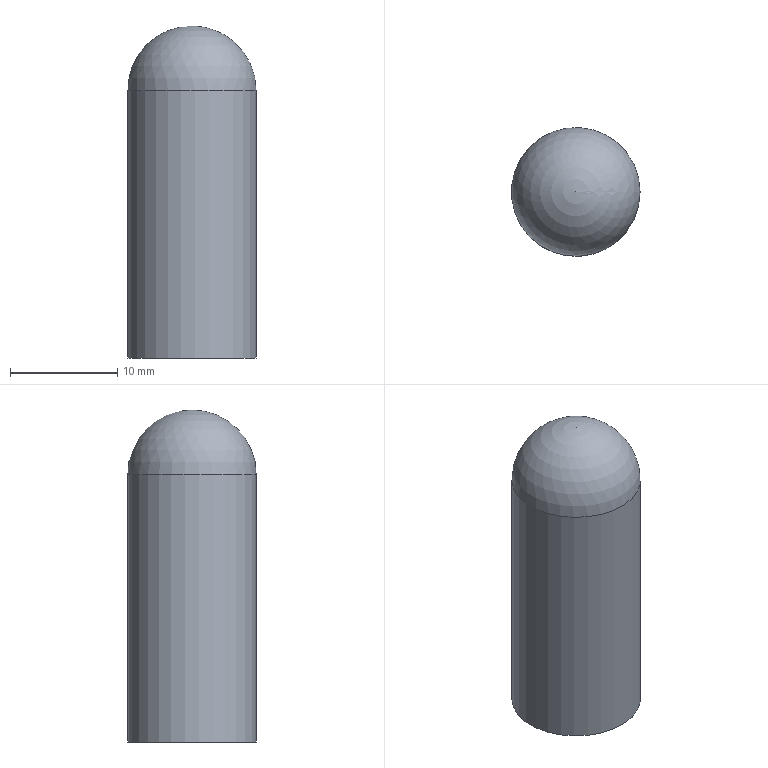Part | NX | features DATUM_CSYS 2, EXTRUDE 1, HOLE PACKAGE 1, SIMPLE HOLE 1, SKETCH 1, SPHERE 1, SYMBOLIC_THREAD 1 | 1 solid | 6 faces | box 12 x 12 x 31 mm | volume 2343 mm3 | cylinder 2 | cone 2 | plane 1 | sphere 1 | commonest cylinder face diameters 6.8 x1 12 x1
STEP:
#1=CARTESIAN_POINT('',(6.,0.,25.));
#2=VERTEX_POINT('',#1);
#3=CARTESIAN_POINT('',(0.,0.,25.));
#4=DIRECTION('',(0.,0.,1.));
#5=DIRECTION('',(1.,0.,0.));
#6=AXIS2_PLACEMENT_3D('',#3,#4,#5);
#7=CIRCLE('',#6,6.);
#8=EDGE_CURVE('',#2,#2,#7,.F.);
#9=ORIENTED_EDGE('',*,*,#8,.T.);
#10=EDGE_LOOP('',(#9));
#11=FACE_BOUND('',#10,.T.);
#12=CARTESIAN_POINT('',(6.,0.,0.));
#13=VERTEX_POINT('',#12);
#14=CARTESIAN_POINT('',(0.,0.,0.));
#15=DIRECTION('',(0.,0.,1.));
#16=DIRECTION('',(1.,0.,0.));
#17=AXIS2_PLACEMENT_3D('',#14,#15,#16);
#18=CIRCLE('',#17,6.);
#19=EDGE_CURVE('',#13,#13,#18,.T.);
#20=ORIENTED_EDGE('',*,*,#19,.T.);
#21=EDGE_LOOP('',(#20));
#22=FACE_BOUND('',#21,.T.);
#23=CARTESIAN_POINT('',(0.,0.,25.));
#24=DIRECTION('',(0.,0.,-1.));
#25=DIRECTION('',(-1.,0.,0.));
#26=AXIS2_PLACEMENT_3D('',#23,#24,#25);
#27=CYLINDRICAL_SURFACE('',#26,6.);
#28=ADVANCED_FACE('',(#11,#22),#27,.T.);
#29=CARTESIAN_POINT('',(4.,0.,0.));
#30=VERTEX_POINT('',#29);
#31=CARTESIAN_POINT('',(0.,0.,0.));
#32=DIRECTION('',(0.,0.,1.));
#33=DIRECTION('',(1.,0.,0.));
#34=AXIS2_PLACEMENT_3D('',#31,#32,#33);
#35=CIRCLE('',#34,4.);
#36=EDGE_CURVE('',#30,#30,#35,.T.);
#37=ORIENTED_EDGE('',*,*,#36,.T.);
#38=EDGE_LOOP('',(#37));
#39=FACE_BOUND('',#38,.T.);
#40=ORIENTED_EDGE('',*,*,#19,.F.);
#41=EDGE_LOOP('',(#40));
#42=FACE_BOUND('',#41,.T.);
#43=CARTESIAN_POINT('',(0.,0.,0.));
#44=DIRECTION('',(0.,0.,1.));
#45=DIRECTION('',(1.,0.,0.));
#46=AXIS2_PLACEMENT_3D('',#43,#44,#45);
#47=PLANE('',#46);
#48=ADVANCED_FACE('',(#39,#42),#47,.F.);
#49=ORIENTED_EDGE('',*,*,#8,.F.);
#50=EDGE_LOOP('',(#49));
#51=FACE_BOUND('',#50,.T.);
#52=CARTESIAN_POINT('',(0.,0.,25.));
#53=DIRECTION('',(0.,0.,1.));
#54=DIRECTION('',(1.,0.,0.));
#55=AXIS2_PLACEMENT_3D('',#52,#53,#54);
#56=SPHERICAL_SURFACE('',#55,6.);
#57=ADVANCED_FACE('',(#51),#56,.T.);
#58=CARTESIAN_POINT('',(3.4,0.,25.));
#59=VERTEX_POINT('',#58);
#60=CARTESIAN_POINT('',(0.,0.,25.));
#61=DIRECTION('',(0.,0.,1.));
#62=DIRECTION('',(1.,0.,0.));
#63=AXIS2_PLACEMENT_3D('',#60,#61,#62);
#64=CIRCLE('',#63,3.4);
#65=EDGE_CURVE('',#59,#59,#64,.F.);
#66=ORIENTED_EDGE('',*,*,#65,.T.);
#67=EDGE_LOOP('',(#66));
#68=FACE_BOUND('',#67,.T.);
#69=CARTESIAN_POINT('',(0.,0.,27.043));
#70=VERTEX_POINT('',#69);
#71=VERTEX_LOOP('',#70);
#72=FACE_BOUND('',#71,.T.);
#73=CARTESIAN_POINT('',(0.,0.,25.));
#74=DIRECTION('',(0.,0.,-1.));
#75=DIRECTION('',(-1.,0.,0.));
#76=AXIS2_PLACEMENT_3D('',#73,#74,#75);
#77=CONICAL_SURFACE('',#76,3.4,1.03);
#78=ADVANCED_FACE('',(#68,#72),#77,.F.);
#79=CARTESIAN_POINT('',(3.4,0.,0.6));
#80=VERTEX_POINT('',#79);
#81=CARTESIAN_POINT('',(0.,0.,0.6));
#82=DIRECTION('',(0.,0.,1.));
#83=DIRECTION('',(1.,0.,0.));
#84=AXIS2_PLACEMENT_3D('',#81,#82,#83);
#85=CIRCLE('',#84,3.4);
#86=EDGE_CURVE('',#80,#80,#85,.F.);
#87=ORIENTED_EDGE('',*,*,#86,.T.);
#88=EDGE_LOOP('',(#87));
#89=FACE_BOUND('',#88,.T.);
#90=ORIENTED_EDGE('',*,*,#65,.F.);
#91=EDGE_LOOP('',(#90));
#92=FACE_BOUND('',#91,.T.);
#93=CARTESIAN_POINT('',(0.,0.,0.));
#94=DIRECTION('',(0.,0.,1.));
#95=DIRECTION('',(1.,0.,0.));
#96=AXIS2_PLACEMENT_3D('',#93,#94,#95);
#97=CYLINDRICAL_SURFACE('',#96,3.4);
#98=ADVANCED_FACE('',(#89,#92),#97,.F.);
#99=ORIENTED_EDGE('',*,*,#86,.F.);
#100=EDGE_LOOP('',(#99));
#101=FACE_BOUND('',#100,.T.);
#102=ORIENTED_EDGE('',*,*,#36,.F.);
#103=EDGE_LOOP('',(#102));
#104=FACE_BOUND('',#103,.T.);
#105=CARTESIAN_POINT('',(0.,0.,0.));
#106=DIRECTION('',(0.,0.,-1.));
#107=DIRECTION('',(-1.,0.,0.));
#108=AXIS2_PLACEMENT_3D('',#105,#106,#107);
#109=CONICAL_SURFACE('',#108,4.,0.7854);
#110=ADVANCED_FACE('',(#101,#104),#109,.F.);
#111=CLOSED_SHELL('',(#28,#48,#57,#78,#98,#110));
#112=MANIFOLD_SOLID_BREP('',#111);
#113=(LENGTH_UNIT()NAMED_UNIT(*)SI_UNIT(.MILLI.,.METRE.));
#114=UNCERTAINTY_MEASURE_WITH_UNIT(LENGTH_MEASURE(0.00001),#113,'','');
#115=(NAMED_UNIT(*)PLANE_ANGLE_UNIT()SI_UNIT($,.RADIAN.));
#116=(NAMED_UNIT(*)SI_UNIT($,.STERADIAN.)SOLID_ANGLE_UNIT());
#117=(GEOMETRIC_REPRESENTATION_CONTEXT(3)GLOBAL_UNCERTAINTY_ASSIGNED_CONTEXT((#114))GLOBAL_UNIT_ASSIGNED_CONTEXT((#113,#115,#116))REPRESENTATION_CONTEXT('',''));
#118=ADVANCED_BREP_SHAPE_REPRESENTATION('',(#112),#117);